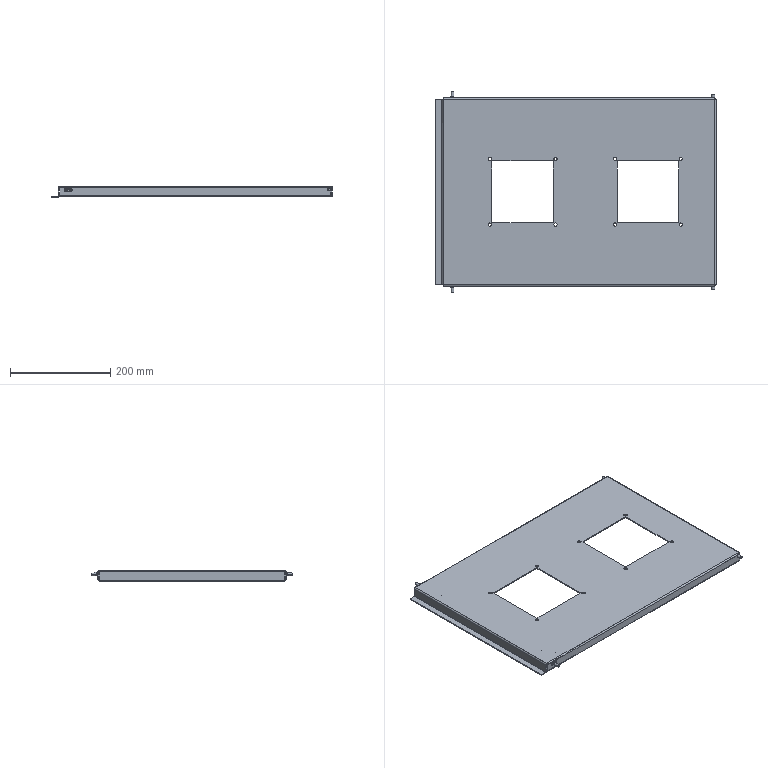Part | SolidWorks | features MoveCopyBody 4, Stock 4, EdgeFlange 3, ICE 2, Cut 1, FlatPattern 1, LPattern 1, SMBaseFlange 1, SheetMetal 1 | 7 solids | 194 faces | box 560 x 402 x 22 mm | volume 485747 mm3 | plane 86 | cylinder 80 | cone 12 | spline 12 | torus 4 | commonest cylinder face diameters 6 x16 6.5 x16 7 x12 11 x12 1.473 x8 5.473 x8